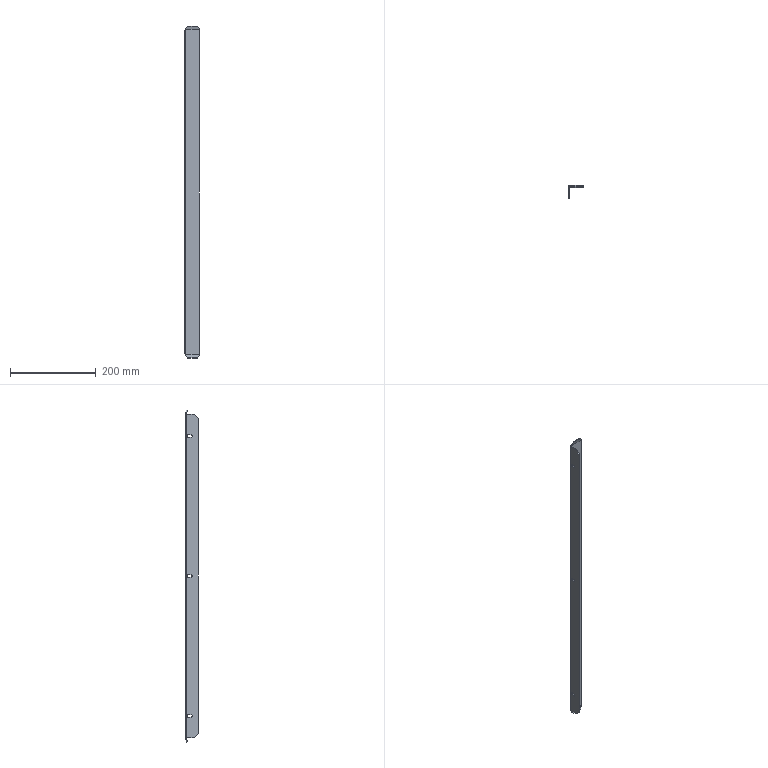Part | STEP file | PN_0005 long bracket plate_Default | 1 solid | 48 faces | box 35 x 30 x 774.978 mm | volume 94609 mm3 | plane 36 | cylinder 12 | commonest cylinder face diameters 6 x6 1.473 x3 5.473 x3